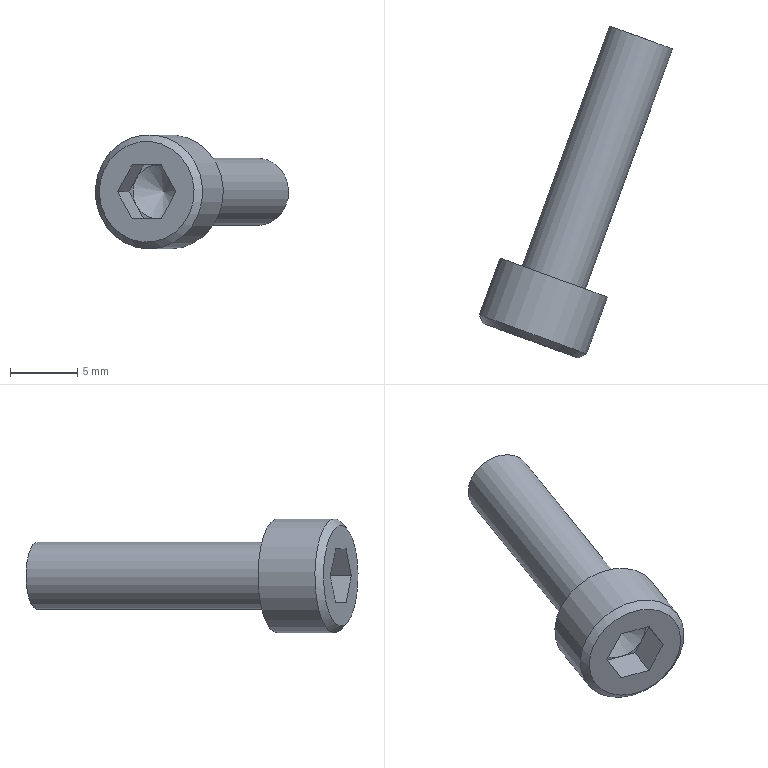Part | NX | features NEZI_5003_007_C-SCPW55-12-15 2 | 1 solid | 19 faces | box 14.38 x 24.69 x 8.5 mm | volume 613.907 mm3 | plane 15 | cone 2 | cylinder 2 | commonest cylinder face diameters 5 x1 8.5 x1
STEP:
#1=CARTESIAN_POINT('',(173.13,-338.436,-315.));
#2=VERTEX_POINT('',#1);
#3=CARTESIAN_POINT('',(172.044,-338.041,-317.));
#4=VERTEX_POINT('',#3);
#5=CARTESIAN_POINT('',(173.13,-338.436,-315.));
#6=DIRECTION('',(-0.4698,0.171,-0.866));
#7=VECTOR('',#6,1000.);
#8=LINE('',#5,#7);
#9=EDGE_CURVE('',#2,#4,#8,.T.);
#10=ORIENTED_EDGE('',*,*,#9,.F.);
#11=CARTESIAN_POINT('',(175.3,-339.226,-315.));
#12=VERTEX_POINT('',#11);
#13=CARTESIAN_POINT('',(175.3,-339.226,-315.));
#14=DIRECTION('',(-0.9397,0.342,0.));
#15=VECTOR('',#14,1000.);
#16=LINE('',#13,#15);
#17=EDGE_CURVE('',#12,#2,#16,.T.);
#18=ORIENTED_EDGE('',*,*,#17,.F.);
#19=CARTESIAN_POINT('',(176.385,-339.621,-317.));
#20=VERTEX_POINT('',#19);
#21=CARTESIAN_POINT('',(176.385,-339.621,-317.));
#22=DIRECTION('',(-0.4698,0.171,0.866));
#23=VECTOR('',#22,1000.);
#24=LINE('',#21,#23);
#25=EDGE_CURVE('',#20,#12,#24,.T.);
#26=ORIENTED_EDGE('',*,*,#25,.F.);
#27=CARTESIAN_POINT('',(175.3,-339.226,-319.));
#28=VERTEX_POINT('',#27);
#29=CARTESIAN_POINT('',(175.3,-339.226,-319.));
#30=DIRECTION('',(0.4698,-0.171,0.866));
#31=VECTOR('',#30,1000.);
#32=LINE('',#29,#31);
#33=EDGE_CURVE('',#28,#20,#32,.T.);
#34=ORIENTED_EDGE('',*,*,#33,.F.);
#35=CARTESIAN_POINT('',(173.13,-338.436,-319.));
#36=VERTEX_POINT('',#35);
#37=CARTESIAN_POINT('',(173.13,-338.436,-319.));
#38=DIRECTION('',(0.9397,-0.342,0.));
#39=VECTOR('',#38,1000.);
#40=LINE('',#37,#39);
#41=EDGE_CURVE('',#36,#28,#40,.T.);
#42=ORIENTED_EDGE('',*,*,#41,.F.);
#43=CARTESIAN_POINT('',(172.044,-338.041,-317.));
#44=DIRECTION('',(0.4698,-0.171,-0.866));
#45=VECTOR('',#44,1000.);
#46=LINE('',#43,#45);
#47=EDGE_CURVE('',#4,#36,#46,.T.);
#48=ORIENTED_EDGE('',*,*,#47,.F.);
#49=EDGE_LOOP('',(#10,#18,#26,#34,#42,#48));
#50=FACE_BOUND('',#49,.T.);
#51=CARTESIAN_POINT('',(177.266,-339.942,-315.125));
#52=VERTEX_POINT('',#51);
#53=CARTESIAN_POINT('',(174.215,-338.831,-317.));
#54=DIRECTION('',(-0.342,-0.9397,0.));
#55=DIRECTION('',(0.8138,-0.2962,0.5));
#56=AXIS2_PLACEMENT_3D('',#53,#54,#55);
#57=CIRCLE('',#56,3.75);
#58=EDGE_CURVE('',#52,#52,#57,.T.);
#59=ORIENTED_EDGE('',*,*,#58,.T.);
#60=EDGE_LOOP('',(#59));
#61=FACE_BOUND('',#60,.T.);
#62=CARTESIAN_POINT('',(174.215,-338.831,-317.));
#63=DIRECTION('',(0.342,0.9397,0.));
#64=DIRECTION('',(-0.8138,0.2962,-0.5));
#65=AXIS2_PLACEMENT_3D('',#62,#63,#64);
#66=PLANE('',#65);
#67=ADVANCED_FACE('',(#50,#61),#66,.F.);
#68=ORIENTED_EDGE('',*,*,#58,.F.);
#69=EDGE_LOOP('',(#68));
#70=FACE_BOUND('',#69,.T.);
#71=CARTESIAN_POINT('',(177.844,-339.62,-314.875));
#72=VERTEX_POINT('',#71);
#73=CARTESIAN_POINT('',(174.386,-338.361,-317.));
#74=DIRECTION('',(-0.342,-0.9397,0.));
#75=DIRECTION('',(0.8138,-0.2962,0.5));
#76=AXIS2_PLACEMENT_3D('',#73,#74,#75);
#77=CIRCLE('',#76,4.25);
#78=EDGE_CURVE('',#72,#72,#77,.T.);
#79=ORIENTED_EDGE('',*,*,#78,.T.);
#80=EDGE_LOOP('',(#79));
#81=FACE_BOUND('',#80,.T.);
#82=CARTESIAN_POINT('',(174.386,-338.361,-317.));
#83=DIRECTION('',(0.342,0.9397,0.));
#84=DIRECTION('',(-0.8138,0.2962,-0.5));
#85=AXIS2_PLACEMENT_3D('',#82,#83,#84);
#86=CONICAL_SURFACE('',#85,4.25,0.7854);
#87=ADVANCED_FACE('',(#70,#81),#86,.T.);
#88=ORIENTED_EDGE('',*,*,#78,.F.);
#89=EDGE_LOOP('',(#88));
#90=FACE_BOUND('',#89,.T.);
#91=CARTESIAN_POINT('',(179.383,-335.392,-314.875));
#92=VERTEX_POINT('',#91);
#93=CARTESIAN_POINT('',(175.925,-334.133,-317.));
#94=DIRECTION('',(-0.342,-0.9397,0.));
#95=DIRECTION('',(0.8138,-0.2962,0.5));
#96=AXIS2_PLACEMENT_3D('',#93,#94,#95);
#97=CIRCLE('',#96,4.25);
#98=EDGE_CURVE('',#92,#92,#97,.T.);
#99=ORIENTED_EDGE('',*,*,#98,.T.);
#100=EDGE_LOOP('',(#99));
#101=FACE_BOUND('',#100,.T.);
#102=CARTESIAN_POINT('',(173.804,-339.959,-317.));
#103=DIRECTION('',(-0.342,-0.9397,0.));
#104=DIRECTION('',(0.8138,-0.2962,0.5));
#105=AXIS2_PLACEMENT_3D('',#102,#103,#104);
#106=CYLINDRICAL_SURFACE('',#105,4.25);
#107=ADVANCED_FACE('',(#90,#101),#106,.T.);
#108=ORIENTED_EDGE('',*,*,#98,.F.);
#109=EDGE_LOOP('',(#108));
#110=FACE_BOUND('',#109,.T.);
#111=CARTESIAN_POINT('',(177.959,-334.873,-315.75));
#112=VERTEX_POINT('',#111);
#113=CARTESIAN_POINT('',(175.925,-334.133,-317.));
#114=DIRECTION('',(-0.342,-0.9397,0.));
#115=DIRECTION('',(0.8138,-0.2962,0.5));
#116=AXIS2_PLACEMENT_3D('',#113,#114,#115);
#117=CIRCLE('',#116,2.5);
#118=EDGE_CURVE('',#112,#112,#117,.T.);
#119=ORIENTED_EDGE('',*,*,#118,.T.);
#120=EDGE_LOOP('',(#119));
#121=FACE_BOUND('',#120,.T.);
#122=CARTESIAN_POINT('',(173.928,-333.406,-313.319));
#123=DIRECTION('',(-0.342,-0.9397,0.));
#124=DIRECTION('',(0.8138,-0.2962,0.5));
#125=AXIS2_PLACEMENT_3D('',#122,#123,#124);
#126=PLANE('',#125);
#127=ADVANCED_FACE('',(#110,#121),#126,.F.);
#128=ORIENTED_EDGE('',*,*,#118,.F.);
#129=EDGE_LOOP('',(#128));
#130=FACE_BOUND('',#129,.T.);
#131=CARTESIAN_POINT('',(184.458,-317.019,-315.75));
#132=VERTEX_POINT('',#131);
#133=CARTESIAN_POINT('',(182.423,-316.279,-317.));
#134=DIRECTION('',(-0.342,-0.9397,0.));
#135=DIRECTION('',(0.8138,-0.2962,0.5));
#136=AXIS2_PLACEMENT_3D('',#133,#134,#135);
#137=CIRCLE('',#136,2.5);
#138=EDGE_CURVE('',#132,#132,#137,.T.);
#139=ORIENTED_EDGE('',*,*,#138,.T.);
#140=EDGE_LOOP('',(#139));
#141=FACE_BOUND('',#140,.T.);
#142=CARTESIAN_POINT('',(173.804,-339.959,-317.));
#143=DIRECTION('',(-0.342,-0.9397,0.));
#144=DIRECTION('',(0.8138,-0.2962,0.5));
#145=AXIS2_PLACEMENT_3D('',#142,#143,#144);
#146=CYLINDRICAL_SURFACE('',#145,2.5);
#147=ADVANCED_FACE('',(#130,#141),#146,.T.);
#148=ORIENTED_EDGE('',*,*,#138,.F.);
#149=EDGE_LOOP('',(#148));
#150=FACE_BOUND('',#149,.T.);
#151=CARTESIAN_POINT('',(181.248,-315.851,-314.835));
#152=DIRECTION('',(-0.342,-0.9397,0.));
#153=DIRECTION('',(0.8138,-0.2962,0.5));
#154=AXIS2_PLACEMENT_3D('',#151,#152,#153);
#155=PLANE('',#154);
#156=ADVANCED_FACE('',(#150),#155,.F.);
#157=ORIENTED_EDGE('',*,*,#17,.T.);
#158=CARTESIAN_POINT('',(173.985,-336.087,-315.));
#159=VERTEX_POINT('',#158);
#160=CARTESIAN_POINT('',(173.985,-336.087,-315.));
#161=DIRECTION('',(-0.342,-0.9397,0.));
#162=VECTOR('',#161,1000.);
#163=LINE('',#160,#162);
#164=EDGE_CURVE('',#159,#2,#163,.T.);
#165=ORIENTED_EDGE('',*,*,#164,.F.);
#166=CARTESIAN_POINT('',(175.07,-336.482,-315.));
#167=VERTEX_POINT('',#166);
#168=CARTESIAN_POINT('',(176.155,-336.877,-315.));
#169=DIRECTION('',(-0.9397,0.342,0.));
#170=VECTOR('',#169,1000.);
#171=LINE('',#168,#170);
#172=EDGE_CURVE('',#167,#159,#171,.T.);
#173=ORIENTED_EDGE('',*,*,#172,.F.);
#174=CARTESIAN_POINT('',(176.155,-336.877,-315.));
#175=VERTEX_POINT('',#174);
#176=CARTESIAN_POINT('',(176.155,-336.877,-315.));
#177=DIRECTION('',(-0.9397,0.342,0.));
#178=VECTOR('',#177,1000.);
#179=LINE('',#176,#178);
#180=EDGE_CURVE('',#175,#167,#179,.T.);
#181=ORIENTED_EDGE('',*,*,#180,.F.);
#182=CARTESIAN_POINT('',(176.155,-336.877,-315.));
#183=DIRECTION('',(-0.342,-0.9397,0.));
#184=VECTOR('',#183,1000.);
#185=LINE('',#182,#184);
#186=EDGE_CURVE('',#175,#12,#185,.T.);
#187=ORIENTED_EDGE('',*,*,#186,.T.);
#188=EDGE_LOOP('',(#157,#165,#173,#181,#187));
#189=FACE_BOUND('',#188,.T.);
#190=CARTESIAN_POINT('',(176.155,-336.877,-315.));
#191=DIRECTION('',(0.,0.,1.));
#192=DIRECTION('',(0.9397,-0.342,0.));
#193=AXIS2_PLACEMENT_3D('',#190,#191,#192);
#194=PLANE('',#193);
#195=ADVANCED_FACE('',(#189),#194,.F.);
#196=ORIENTED_EDGE('',*,*,#25,.T.);
#197=ORIENTED_EDGE('',*,*,#186,.F.);
#198=CARTESIAN_POINT('',(176.697,-337.074,-316.));
#199=VERTEX_POINT('',#198);
#200=CARTESIAN_POINT('',(177.24,-337.272,-317.));
#201=DIRECTION('',(-0.4698,0.171,0.866));
#202=VECTOR('',#201,1000.);
#203=LINE('',#200,#202);
#204=EDGE_CURVE('',#199,#175,#203,.T.);
#205=ORIENTED_EDGE('',*,*,#204,.F.);
#206=CARTESIAN_POINT('',(177.24,-337.272,-317.));
#207=VERTEX_POINT('',#206);
#208=CARTESIAN_POINT('',(177.24,-337.272,-317.));
#209=DIRECTION('',(-0.4698,0.171,0.866));
#210=VECTOR('',#209,1000.);
#211=LINE('',#208,#210);
#212=EDGE_CURVE('',#207,#199,#211,.T.);
#213=ORIENTED_EDGE('',*,*,#212,.F.);
#214=CARTESIAN_POINT('',(177.24,-337.272,-317.));
#215=DIRECTION('',(-0.342,-0.9397,0.));
#216=VECTOR('',#215,1000.);
#217=LINE('',#214,#216);
#218=EDGE_CURVE('',#207,#20,#217,.T.);
#219=ORIENTED_EDGE('',*,*,#218,.T.);
#220=EDGE_LOOP('',(#196,#197,#205,#213,#219));
#221=FACE_BOUND('',#220,.T.);
#222=CARTESIAN_POINT('',(177.24,-337.272,-317.));
#223=DIRECTION('',(0.8138,-0.2962,0.5));
#224=DIRECTION('',(0.4698,-0.171,-0.866));
#225=AXIS2_PLACEMENT_3D('',#222,#223,#224);
#226=PLANE('',#225);
#227=ADVANCED_FACE('',(#221),#226,.F.);
#228=ORIENTED_EDGE('',*,*,#33,.T.);
#229=ORIENTED_EDGE('',*,*,#218,.F.);
#230=CARTESIAN_POINT('',(176.697,-337.074,-318.));
#231=VERTEX_POINT('',#230);
#232=CARTESIAN_POINT('',(176.155,-336.877,-319.));
#233=DIRECTION('',(0.4698,-0.171,0.866));
#234=VECTOR('',#233,1000.);
#235=LINE('',#232,#234);
#236=EDGE_CURVE('',#231,#207,#235,.T.);
#237=ORIENTED_EDGE('',*,*,#236,.F.);
#238=CARTESIAN_POINT('',(176.155,-336.877,-319.));
#239=VERTEX_POINT('',#238);
#240=CARTESIAN_POINT('',(176.155,-336.877,-319.));
#241=DIRECTION('',(0.4698,-0.171,0.866));
#242=VECTOR('',#241,1000.);
#243=LINE('',#240,#242);
#244=EDGE_CURVE('',#239,#231,#243,.T.);
#245=ORIENTED_EDGE('',*,*,#244,.F.);
#246=CARTESIAN_POINT('',(176.155,-336.877,-319.));
#247=DIRECTION('',(-0.342,-0.9397,0.));
#248=VECTOR('',#247,1000.);
#249=LINE('',#246,#248);
#250=EDGE_CURVE('',#239,#28,#249,.T.);
#251=ORIENTED_EDGE('',*,*,#250,.T.);
#252=EDGE_LOOP('',(#228,#229,#237,#245,#251));
#253=FACE_BOUND('',#252,.T.);
#254=CARTESIAN_POINT('',(176.155,-336.877,-319.));
#255=DIRECTION('',(0.8138,-0.2962,-0.5));
#256=DIRECTION('',(-0.4698,0.171,-0.866));
#257=AXIS2_PLACEMENT_3D('',#254,#255,#256);
#258=PLANE('',#257);
#259=ADVANCED_FACE('',(#253),#258,.F.);
#260=ORIENTED_EDGE('',*,*,#41,.T.);
#261=ORIENTED_EDGE('',*,*,#250,.F.);
#262=CARTESIAN_POINT('',(175.07,-336.482,-319.));
#263=VERTEX_POINT('',#262);
#264=CARTESIAN_POINT('',(173.985,-336.087,-319.));
#265=DIRECTION('',(0.9397,-0.342,0.));
#266=VECTOR('',#265,1000.);
#267=LINE('',#264,#266);
#268=EDGE_CURVE('',#263,#239,#267,.T.);
#269=ORIENTED_EDGE('',*,*,#268,.F.);
#270=CARTESIAN_POINT('',(173.985,-336.087,-319.));
#271=VERTEX_POINT('',#270);
#272=CARTESIAN_POINT('',(173.985,-336.087,-319.));
#273=DIRECTION('',(0.9397,-0.342,0.));
#274=VECTOR('',#273,1000.);
#275=LINE('',#272,#274);
#276=EDGE_CURVE('',#271,#263,#275,.T.);
#277=ORIENTED_EDGE('',*,*,#276,.F.);
#278=CARTESIAN_POINT('',(173.985,-336.087,-319.));
#279=DIRECTION('',(-0.342,-0.9397,0.));
#280=VECTOR('',#279,1000.);
#281=LINE('',#278,#280);
#282=EDGE_CURVE('',#271,#36,#281,.T.);
#283=ORIENTED_EDGE('',*,*,#282,.T.);
#284=EDGE_LOOP('',(#260,#261,#269,#277,#283));
#285=FACE_BOUND('',#284,.T.);
#286=CARTESIAN_POINT('',(173.985,-336.087,-319.));
#287=DIRECTION('',(0.,0.,-1.));
#288=DIRECTION('',(-0.9397,0.342,0.));
#289=AXIS2_PLACEMENT_3D('',#286,#287,#288);
#290=PLANE('',#289);
#291=ADVANCED_FACE('',(#285),#290,.F.);
#292=ORIENTED_EDGE('',*,*,#47,.T.);
#293=ORIENTED_EDGE('',*,*,#282,.F.);
#294=CARTESIAN_POINT('',(173.442,-335.89,-318.));
#295=VERTEX_POINT('',#294);
#296=CARTESIAN_POINT('',(172.9,-335.692,-317.));
#297=DIRECTION('',(0.4698,-0.171,-0.866));
#298=VECTOR('',#297,1000.);
#299=LINE('',#296,#298);
#300=EDGE_CURVE('',#295,#271,#299,.T.);
#301=ORIENTED_EDGE('',*,*,#300,.F.);
#302=CARTESIAN_POINT('',(172.9,-335.692,-317.));
#303=VERTEX_POINT('',#302);
#304=CARTESIAN_POINT('',(172.9,-335.692,-317.));
#305=DIRECTION('',(0.4698,-0.171,-0.866));
#306=VECTOR('',#305,1000.);
#307=LINE('',#304,#306);
#308=EDGE_CURVE('',#303,#295,#307,.T.);
#309=ORIENTED_EDGE('',*,*,#308,.F.);
#310=CARTESIAN_POINT('',(172.9,-335.692,-317.));
#311=DIRECTION('',(-0.342,-0.9397,0.));
#312=VECTOR('',#311,1000.);
#313=LINE('',#310,#312);
#314=EDGE_CURVE('',#303,#4,#313,.T.);
#315=ORIENTED_EDGE('',*,*,#314,.T.);
#316=EDGE_LOOP('',(#292,#293,#301,#309,#315));
#317=FACE_BOUND('',#316,.T.);
#318=CARTESIAN_POINT('',(172.9,-335.692,-317.));
#319=DIRECTION('',(-0.8138,0.2962,-0.5));
#320=DIRECTION('',(-0.342,-0.9397,0.));
#321=AXIS2_PLACEMENT_3D('',#318,#319,#320);
#322=PLANE('',#321);
#323=ADVANCED_FACE('',(#317),#322,.F.);
#324=ORIENTED_EDGE('',*,*,#9,.T.);
#325=ORIENTED_EDGE('',*,*,#314,.F.);
#326=CARTESIAN_POINT('',(173.442,-335.89,-316.));
#327=VERTEX_POINT('',#326);
#328=CARTESIAN_POINT('',(173.985,-336.087,-315.));
#329=DIRECTION('',(-0.4698,0.171,-0.866));
#330=VECTOR('',#329,1000.);
#331=LINE('',#328,#330);
#332=EDGE_CURVE('',#327,#303,#331,.T.);
#333=ORIENTED_EDGE('',*,*,#332,.F.);
#334=CARTESIAN_POINT('',(173.985,-336.087,-315.));
#335=DIRECTION('',(-0.4698,0.171,-0.866));
#336=VECTOR('',#335,1000.);
#337=LINE('',#334,#336);
#338=EDGE_CURVE('',#159,#327,#337,.T.);
#339=ORIENTED_EDGE('',*,*,#338,.F.);
#340=ORIENTED_EDGE('',*,*,#164,.T.);
#341=EDGE_LOOP('',(#324,#325,#333,#339,#340));
#342=FACE_BOUND('',#341,.T.);
#343=CARTESIAN_POINT('',(173.985,-336.087,-315.));
#344=DIRECTION('',(-0.8138,0.2962,0.5));
#345=DIRECTION('',(0.4698,-0.171,0.866));
#346=AXIS2_PLACEMENT_3D('',#343,#344,#345);
#347=PLANE('',#346);
#348=ADVANCED_FACE('',(#342),#347,.F.);
#349=CARTESIAN_POINT('',(175.07,-336.482,-317.));
#350=DIRECTION('',(-0.342,-0.9397,0.));
#351=DIRECTION('',(0.8138,-0.2962,0.5));
#352=AXIS2_PLACEMENT_3D('',#349,#350,#351);
#353=CIRCLE('',#352,2.);
#354=EDGE_CURVE('',#231,#199,#353,.T.);
#355=ORIENTED_EDGE('',*,*,#354,.F.);
#356=ORIENTED_EDGE('',*,*,#236,.T.);
#357=ORIENTED_EDGE('',*,*,#212,.T.);
#358=EDGE_LOOP('',(#355,#356,#357));
#359=FACE_BOUND('',#358,.T.);
#360=CARTESIAN_POINT('',(175.07,-336.482,-317.));
#361=DIRECTION('',(-0.342,-0.9397,0.));
#362=DIRECTION('',(0.8138,-0.2962,0.5));
#363=AXIS2_PLACEMENT_3D('',#360,#361,#362);
#364=PLANE('',#363);
#365=ADVANCED_FACE('',(#359),#364,.T.);
#366=CARTESIAN_POINT('',(175.07,-336.482,-317.));
#367=DIRECTION('',(-0.342,-0.9397,0.));
#368=DIRECTION('',(0.8138,-0.2962,0.5));
#369=AXIS2_PLACEMENT_3D('',#366,#367,#368);
#370=CIRCLE('',#369,2.);
#371=EDGE_CURVE('',#263,#231,#370,.T.);
#372=ORIENTED_EDGE('',*,*,#371,.F.);
#373=ORIENTED_EDGE('',*,*,#268,.T.);
#374=ORIENTED_EDGE('',*,*,#244,.T.);
#375=EDGE_LOOP('',(#372,#373,#374));
#376=FACE_BOUND('',#375,.T.);
#377=CARTESIAN_POINT('',(175.07,-336.482,-317.));
#378=DIRECTION('',(-0.342,-0.9397,0.));
#379=DIRECTION('',(0.8138,-0.2962,0.5));
#380=AXIS2_PLACEMENT_3D('',#377,#378,#379);
#381=PLANE('',#380);
#382=ADVANCED_FACE('',(#376),#381,.T.);
#383=CARTESIAN_POINT('',(175.07,-336.482,-317.));
#384=DIRECTION('',(-0.342,-0.9397,0.));
#385=DIRECTION('',(0.8138,-0.2962,0.5));
#386=AXIS2_PLACEMENT_3D('',#383,#384,#385);
#387=CIRCLE('',#386,2.);
#388=EDGE_CURVE('',#295,#263,#387,.T.);
#389=ORIENTED_EDGE('',*,*,#388,.F.);
#390=ORIENTED_EDGE('',*,*,#300,.T.);
#391=ORIENTED_EDGE('',*,*,#276,.T.);
#392=EDGE_LOOP('',(#389,#390,#391));
#393=FACE_BOUND('',#392,.T.);
#394=CARTESIAN_POINT('',(175.07,-336.482,-317.));
#395=DIRECTION('',(-0.342,-0.9397,0.));
#396=DIRECTION('',(0.8138,-0.2962,0.5));
#397=AXIS2_PLACEMENT_3D('',#394,#395,#396);
#398=PLANE('',#397);
#399=ADVANCED_FACE('',(#393),#398,.T.);
#400=CARTESIAN_POINT('',(175.07,-336.482,-317.));
#401=DIRECTION('',(-0.342,-0.9397,0.));
#402=DIRECTION('',(0.8138,-0.2962,0.5));
#403=AXIS2_PLACEMENT_3D('',#400,#401,#402);
#404=CIRCLE('',#403,2.);
#405=EDGE_CURVE('',#327,#295,#404,.T.);
#406=ORIENTED_EDGE('',*,*,#405,.F.);
#407=ORIENTED_EDGE('',*,*,#332,.T.);
#408=ORIENTED_EDGE('',*,*,#308,.T.);
#409=EDGE_LOOP('',(#406,#407,#408));
#410=FACE_BOUND('',#409,.T.);
#411=CARTESIAN_POINT('',(175.07,-336.482,-317.));
#412=DIRECTION('',(-0.342,-0.9397,0.));
#413=DIRECTION('',(0.8138,-0.2962,0.5));
#414=AXIS2_PLACEMENT_3D('',#411,#412,#413);
#415=PLANE('',#414);
#416=ADVANCED_FACE('',(#410),#415,.T.);
#417=CARTESIAN_POINT('',(175.07,-336.482,-317.));
#418=DIRECTION('',(-0.342,-0.9397,0.));
#419=DIRECTION('',(0.8138,-0.2962,0.5));
#420=AXIS2_PLACEMENT_3D('',#417,#418,#419);
#421=CIRCLE('',#420,2.);
#422=EDGE_CURVE('',#167,#327,#421,.T.);
#423=ORIENTED_EDGE('',*,*,#422,.F.);
#424=ORIENTED_EDGE('',*,*,#172,.T.);
#425=ORIENTED_EDGE('',*,*,#338,.T.);
#426=EDGE_LOOP('',(#423,#424,#425));
#427=FACE_BOUND('',#426,.T.);
#428=CARTESIAN_POINT('',(175.07,-336.482,-317.));
#429=DIRECTION('',(-0.342,-0.9397,0.));
#430=DIRECTION('',(0.8138,-0.2962,0.5));
#431=AXIS2_PLACEMENT_3D('',#428,#429,#430);
#432=PLANE('',#431);
#433=ADVANCED_FACE('',(#427),#432,.T.);
#434=CARTESIAN_POINT('',(175.07,-336.482,-317.));
#435=DIRECTION('',(-0.342,-0.9397,0.));
#436=DIRECTION('',(0.8138,-0.2962,0.5));
#437=AXIS2_PLACEMENT_3D('',#434,#435,#436);
#438=CIRCLE('',#437,2.);
#439=EDGE_CURVE('',#199,#167,#438,.T.);
#440=ORIENTED_EDGE('',*,*,#439,.F.);
#441=ORIENTED_EDGE('',*,*,#204,.T.);
#442=ORIENTED_EDGE('',*,*,#180,.T.);
#443=EDGE_LOOP('',(#440,#441,#442));
#444=FACE_BOUND('',#443,.T.);
#445=CARTESIAN_POINT('',(175.07,-336.482,-317.));
#446=DIRECTION('',(-0.342,-0.9397,0.));
#447=DIRECTION('',(0.8138,-0.2962,0.5));
#448=AXIS2_PLACEMENT_3D('',#445,#446,#447);
#449=PLANE('',#448);
#450=ADVANCED_FACE('',(#444),#449,.T.);
#451=CARTESIAN_POINT('',(175.481,-335.353,-317.));
#452=VERTEX_POINT('',#451);
#453=VERTEX_LOOP('',#452);
#454=FACE_BOUND('',#453,.T.);
#455=ORIENTED_EDGE('',*,*,#439,.T.);
#456=ORIENTED_EDGE('',*,*,#422,.T.);
#457=ORIENTED_EDGE('',*,*,#405,.T.);
#458=ORIENTED_EDGE('',*,*,#388,.T.);
#459=ORIENTED_EDGE('',*,*,#371,.T.);
#460=ORIENTED_EDGE('',*,*,#354,.T.);
#461=EDGE_LOOP('',(#455,#456,#457,#458,#459,#460));
#462=FACE_BOUND('',#461,.T.);
#463=CARTESIAN_POINT('',(175.07,-336.482,-317.));
#464=DIRECTION('',(-0.342,-0.9397,0.));
#465=DIRECTION('',(0.8138,-0.2962,0.5));
#466=AXIS2_PLACEMENT_3D('',#463,#464,#465);
#467=CONICAL_SURFACE('',#466,2.,1.03);
#468=ADVANCED_FACE('',(#454,#462),#467,.F.);
#469=CLOSED_SHELL('',(#67,#87,#107,#127,#147,#156,#195,#227,#259,#291,#323,#348,#365,#382,#399,#416,#433,#450,#468));
#470=MANIFOLD_SOLID_BREP('',#469);
#471=(LENGTH_UNIT()NAMED_UNIT(*)SI_UNIT(.MILLI.,.METRE.));
#472=UNCERTAINTY_MEASURE_WITH_UNIT(LENGTH_MEASURE(0.00001),#471,'','');
#473=(NAMED_UNIT(*)PLANE_ANGLE_UNIT()SI_UNIT($,.RADIAN.));
#474=(NAMED_UNIT(*)SI_UNIT($,.STERADIAN.)SOLID_ANGLE_UNIT());
#475=(GEOMETRIC_REPRESENTATION_CONTEXT(3)GLOBAL_UNCERTAINTY_ASSIGNED_CONTEXT((#472))GLOBAL_UNIT_ASSIGNED_CONTEXT((#471,#473,#474))REPRESENTATION_CONTEXT('',''));
#476=ADVANCED_BREP_SHAPE_REPRESENTATION('',(#470),#475);